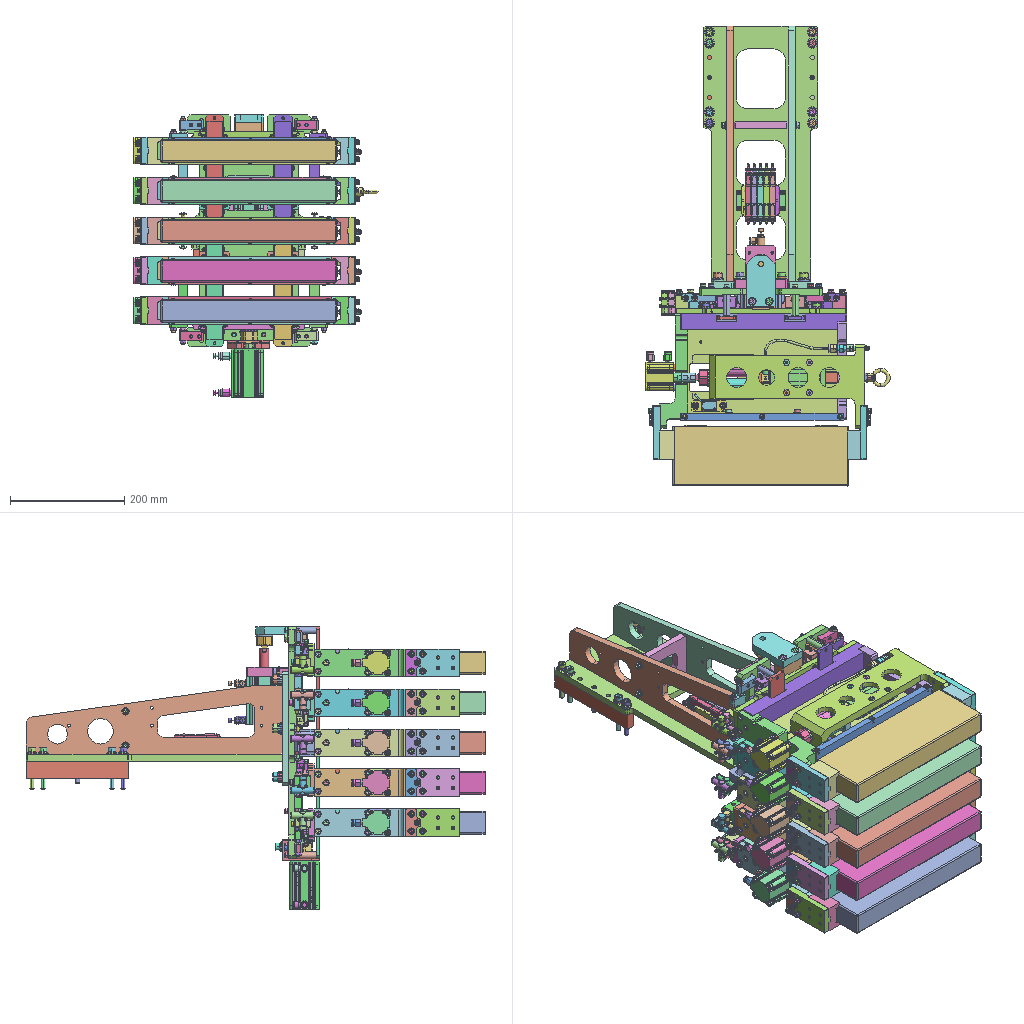Assembly | STEP file | 1222 different items | 1222 placed | box 427 x 805 x 495 mm
Parts list (item | name | quantity | parent item | size | volume), first 273 of 1222 items:
1 | 25A-CDQ2B32-15DZ-M9BWSDPC-Part-1 | x1 | in 25A-CDQ2B32-15DZ-M9BWSDPC | 27 x 4 x 4.6 mm | 354.995 mm3
2 | 25A-CDQ2B32-15DZ-M9BWSDPC-Part-1-1 | x1 | in 25A-CDQ2B32-15DZ-M9BWSDPC-1 | 27 x 4 x 4.6 mm | 354.995 mm3
3 | 25A-CDQ2B32-15DZ-M9BWSDPC-Part-1-2 | x1 | in 25A-CDQ2B32-15DZ-M9BWSDPC-2 | 27 x 4 x 4.6 mm | 354.995 mm3
4 | 25A-CDQ2B32-15DZ-M9BWSDPC-Part-1-3 | x1 | in 25A-CDQ2B32-15DZ-M9BWSDPC-3 | 27 x 4 x 4.6 mm | 354.995 mm3
5 | 25A-CDQ2B32-15DZ-M9BWSDPC-Part-1-4 | x1 | in 25A-CDQ2B32-15DZ-M9BWSDPC-4 | 27 x 4 x 4.6 mm | 354.995 mm3
6 | 25A-CDQ2B32-15DZ-M9BWSDPC-Part-2 | x1 | in 25A-CDQ2B32-15DZ-M9BWSDPC | 48 x 45 x 49.5 mm | 58108 mm3
7 | 25A-CDQ2B32-15DZ-M9BWSDPC-Part-2-1 | x1 | in 25A-CDQ2B32-15DZ-M9BWSDPC-1 | 48 x 45 x 49.5 mm | 58108 mm3
8 | 25A-CDQ2B32-15DZ-M9BWSDPC-Part-2-2 | x1 | in 25A-CDQ2B32-15DZ-M9BWSDPC-2 | 48 x 45 x 49.5 mm | 58108 mm3
9 | 25A-CDQ2B32-15DZ-M9BWSDPC-Part-2-3 | x1 | in 25A-CDQ2B32-15DZ-M9BWSDPC-3 | 48 x 45 x 49.5 mm | 58108 mm3
10 | 25A-CDQ2B32-15DZ-M9BWSDPC-Part-2-4 | x1 | in 25A-CDQ2B32-15DZ-M9BWSDPC-4 | 48 x 45 x 49.5 mm | 58108 mm3
11 | 25A-CDQ2B32-15DZ-M9BWSDPC-Part-3 | x1 | in 25A-CDQ2B32-15DZ-M9BWSDPC | 27 x 4 x 4.6 mm | 354.995 mm3
12 | 25A-CDQ2B32-15DZ-M9BWSDPC-Part-3-1 | x1 | in 25A-CDQ2B32-15DZ-M9BWSDPC-1 | 27 x 4 x 4.6 mm | 354.995 mm3
13 | 25A-CDQ2B32-15DZ-M9BWSDPC-Part-3-2 | x1 | in 25A-CDQ2B32-15DZ-M9BWSDPC-2 | 27 x 4 x 4.6 mm | 354.995 mm3
14 | 25A-CDQ2B32-15DZ-M9BWSDPC-Part-3-3 | x1 | in 25A-CDQ2B32-15DZ-M9BWSDPC-3 | 27 x 4 x 4.6 mm | 354.995 mm3
15 | 25A-CDQ2B32-15DZ-M9BWSDPC-Part-3-4 | x1 | in 25A-CDQ2B32-15DZ-M9BWSDPC-4 | 27 x 4 x 4.6 mm | 354.995 mm3
16 | 25A-CDQ2B40-45DZ-M9BWSDPC-Part-1 | x1 | in 25A-CDQ2B40-45DZ-M9BWSDPC | 84.5 x 52 x 57 mm | 122749 mm3
17 | 25A-CDQ2B40-45DZ-M9BWSDPC-Part-1-1 | x1 | in 25A-CDQ2B40-45DZ-M9BWSDPC-1 | 27 x 4 x 4.6 mm | 354.995 mm3
18 | 25A-CDQ2B40-45DZ-M9BWSDPC-Part-2 | x1 | in 25A-CDQ2B40-45DZ-M9BWSDPC | 27 x 4 x 4.6 mm | 354.995 mm3
19 | 25A-CDQ2B40-45DZ-M9BWSDPC-Part-2-1 | x1 | in 25A-CDQ2B40-45DZ-M9BWSDPC-1 | 27 x 4 x 4.6 mm | 354.995 mm3
20 | 25A-CDQ2B40-45DZ-M9BWSDPC-Part-3 | x1 | in 25A-CDQ2B40-45DZ-M9BWSDPC | 27 x 4 x 4.6 mm | 354.995 mm3
21 | 25A-CDQ2B40-45DZ-M9BWSDPC-Part-3-1 | x1 | in 25A-CDQ2B40-45DZ-M9BWSDPC-1 | 84.5 x 52 x 57 mm | 122749 mm3
22 | AS2002FG-06A | x1 | in elevator8 | 12.3 x 31.4 x 43.1 mm | 6190 mm3
23 | AS2002FG-06A-1 | x1 | in elevator8 | 12.3 x 31.4 x 43.1 mm | 6190 mm3
24 | AS2002FG-06A-2 | x1 | in elevator8 | 12.3 x 31.4 x 43.1 mm | 6190 mm3
25 | AS2002FG-06A-3 | x1 | in elevator8 | 12.3 x 31.4 x 43.1 mm | 6190 mm3
26 | AS2002FG-06A-4 | x1 | in elevator8 | 12.3 x 31.4 x 43.1 mm | 6190 mm3
27 | AS2002FG-06A-5 | x1 | in elevator8 | 12.3 x 31.4 x 43.1 mm | 6190 mm3
28 | AS2002FG-06A-6 | x1 | in elevator8 | 12.3 x 31.4 x 43.1 mm | 6190 mm3
29 | AS2002FG-06A-7 | x1 | in elevator8 | 12.3 x 31.4 x 43.1 mm | 6190 mm3
30 | AS2002FG-06A-8 | x1 | in elevator8 | 12.3 x 31.4 x 43.1 mm | 6190 mm3
31 | AS2002FG-06A-9 | x1 | in elevator8 | 12.3 x 31.4 x 43.1 mm | 6190 mm3
32 | AS2201FG-01-06S | x1 | in elevator8 | 14.2 x 35.2 x 27.5 mm | 4200 mm3
33 | AS2201FG-01-06S-1 | x1 | in elevator8 | 14.2 x 35.2 x 27.5 mm | 4200 mm3
34 | AS2201FG-01-06S-2 | x1 | in elevator8 | 14.2 x 35.2 x 27.5 mm | 4200 mm3
35 | AS2201FG-01-06S-3 | x1 | in elevator8 | 14.2 x 35.2 x 27.5 mm | 4200 mm3
36 | B-1132-8 | x1 | in elevator8 | 32.6 x 39.3 x 16 mm | 3782 mm3
37 | BB62-M10-30L | x1 | in J454-EBZ05-02-00 | 16 x 40 x 16 mm | 3957 mm3
38 | BB62-M10-30L-1 | x1 | in J454-EBZ05-02-00 | 16 x 40 x 16 mm | 3957 mm3
39 | BB62-M10-30L-2 | x1 | in J454-EBZ05-02-00 | 16 x 40 x 16 mm | 3957 mm3
40 | BB62-M10-30L-3 | x1 | in J454-EBZ05-02-00 | 16 x 40 x 16 mm | 3957 mm3
41 | BB62-M10-30L-4 | x1 | in J454-EBZ05-02-00 | 16 x 40 x 16 mm | 3957 mm3
42 | BB62-M10-30L-5 | x1 | in J454-EBZ05-02-00 | 16 x 40 x 16 mm | 3957 mm3
43 | BB62-M3-30L | x1 | in elevator8 | 5.5 x 33 x 5.5 mm | 272.045 mm3
44 | BB62-M3-30L-1 | x1 | in elevator8 | 5.5 x 33 x 5.5 mm | 272.045 mm3
45 | BB62-M3-30L-2 | x1 | in elevator8 | 5.5 x 33 x 5.5 mm | 272.045 mm3
46 | BB62-M3-30L-3 | x1 | in elevator8 | 5.5 x 33 x 5.5 mm | 272.045 mm3
47 | BB62-M3-30L-4 | x1 | in elevator8 | 5.5 x 33 x 5.5 mm | 272.045 mm3
48 | BB62-M3-30L-5 | x1 | in elevator8 | 5.5 x 33 x 5.5 mm | 272.045 mm3
49 | BB62-M3-30L-6 | x1 | in elevator8 | 5.5 x 33 x 5.5 mm | 272.045 mm3
50 | BB62-M3-30L-7 | x1 | in elevator8 | 5.5 x 33 x 5.5 mm | 272.045 mm3
51 | BB62-M3-40L | x1 | in elevator8 | 5.5 x 43 x 5.5 mm | 342.731 mm3
52 | BB62-M3-40L-1 | x1 | in elevator8 | 5.5 x 43 x 5.5 mm | 342.731 mm3
53 | BB62-M3-8L | x1 | in J454-EBZ05-18-00 | 5.5 x 11 x 5.5 mm | 116.536 mm3
54 | BB62-M3-8L-1 | x1 | in J454-EBZ05-18-00 | 5.5 x 11 x 5.5 mm | 116.536 mm3
55 | BB62-M3-8L-2 | x1 | in J454-EBZ05-18-00-1 | 5.5 x 11 x 5.5 mm | 116.536 mm3
56 | BB62-M3-8L-3 | x1 | in J454-EBZ05-18-00-1 | 5.5 x 11 x 5.5 mm | 116.536 mm3
57 | BB62-M3-8L-4 | x1 | in J454-EBZ05-18-00-2 | 5.5 x 11 x 5.5 mm | 116.536 mm3
58 | BB62-M3-8L-5 | x1 | in J454-EBZ05-18-00-2 | 5.5 x 11 x 5.5 mm | 116.536 mm3
59 | BB62-M3-8L-6 | x1 | in J454-EBZ05-18-00-3 | 5.5 x 11 x 5.5 mm | 116.536 mm3
60 | BB62-M3-8L-7 | x1 | in J454-EBZ05-18-00-3 | 5.5 x 11 x 5.5 mm | 116.536 mm3
61 | BB62-M3-8L-8 | x1 | in J454-EBZ05-18-00-4 | 5.5 x 11 x 5.5 mm | 116.536 mm3
62 | BB62-M3-8L-9 | x1 | in J454-EBZ05-18-00-4 | 5.5 x 11 x 5.5 mm | 116.536 mm3
63 | BB62-M4-12L | x1 | in J454-EBZ05-01-04 | 7 x 16 x 7 mm | 280.182 mm3
64 | BB62-M4-12L-1 | x1 | in J454-EBZ05-01-04 | 7 x 16 x 7 mm | 280.182 mm3
65 | BB62-M4-8L | x1 | in J454-EBZ05-37-04 | 7 x 12 x 7 mm | 229.916 mm3
66 | BB62-M4-8L-1 | x1 | in J454-EBZ05-37-04-1 | 7 x 12 x 7 mm | 229.916 mm3
67 | BB62-M4-8L-2 | x1 | in J454-EBZ05-37-04-2 | 7 x 12 x 7 mm | 229.916 mm3
68 | BB62-M4-8L-3 | x1 | in J454-EBZ05-37-04-3 | 7 x 12 x 7 mm | 229.916 mm3
69 | BB62-M4-8L-4 | x1 | in J454-EBZ05-37-04-4 | 7 x 12 x 7 mm | 229.916 mm3
70 | BB62-M4-8L-5 | x1 | in J454-EBZ05-37-04-5 | 7 x 12 x 7 mm | 229.916 mm3
71 | BB62-M4-8L-6 | x1 | in J454-EBZ05-37-04-6 | 7 x 12 x 7 mm | 229.916 mm3
72 | BB62-M4-8L-7 | x1 | in J454-EBZ05-37-04-7 | 7 x 12 x 7 mm | 229.916 mm3
73 | BB62-M4-8L-8 | x1 | in J454-EBZ05-37-04-8 | 7 x 12 x 7 mm | 229.916 mm3
74 | BB62-M4-8L-9 | x1 | in J454-EBZ05-37-04-9 | 7 x 12 x 7 mm | 229.916 mm3
75 | BB62-M5-12L | x1 | in J454-EBZ05-06-00 | 8.5 x 17 x 8.5 mm | 467.118 mm3
76 | BB62-M5-12L-1 | x1 | in J454-EBZ05-06-00 | 8.5 x 17 x 8.5 mm | 467.118 mm3
77 | BB62-M5-12L-2 | x1 | in J454-EBZ05-06-00 | 8.5 x 17 x 8.5 mm | 467.118 mm3
78 | BB62-M5-12L-3 | x1 | in J454-EBZ05-06-00 | 8.5 x 17 x 8.5 mm | 467.118 mm3
79 | BB62-M5-12L-4 | x1 | in J454-EBZ05-06-00 | 8.5 x 17 x 8.5 mm | 467.118 mm3
80 | BB62-M5-12L-5 | x1 | in J454-EBZ05-06-00 | 8.5 x 17 x 8.5 mm | 467.118 mm3
81 | BB62-M5-12L-6 | x1 | in J454-EBZ05-06-00 | 8.5 x 17 x 8.5 mm | 467.118 mm3
82 | BB62-M5-12L-7 | x1 | in J454-EBZ05-06-00 | 8.5 x 17 x 8.5 mm | 467.118 mm3
83 | BB62-M5-15L | x1 | in J454-EBZ05-17-00 | 8.5 x 20 x 8.5 mm | 526.023 mm3
84 | BB62-M5-15L-1 | x1 | in J454-EBZ05-17-00-1 | 8.5 x 20 x 8.5 mm | 526.023 mm3
85 | BB62-M5-15L-10 | x1 | in J454-EBZ05-12-03 | 8.5 x 20 x 8.5 mm | 526.023 mm3
86 | BB62-M5-15L-11 | x1 | in J454-EBZ05-17-00-2 | 8.5 x 20 x 8.5 mm | 526.023 mm3
87 | BB62-M5-15L-12 | x1 | in J454-EBZ05-17-00-3 | 8.5 x 20 x 8.5 mm | 526.023 mm3
88 | BB62-M5-15L-13 | x1 | in J454-EBZ05-17-00-4 | 8.5 x 20 x 8.5 mm | 526.023 mm3
89 | BB62-M5-15L-14 | x1 | in J454-EBZ05-17-00-5 | 8.5 x 20 x 8.5 mm | 526.023 mm3
90 | BB62-M5-15L-15 | x1 | in J454-EBZ05-12-03-1 | 8.5 x 20 x 8.5 mm | 526.023 mm3
91 | BB62-M5-15L-16 | x1 | in J454-EBZ05-12-03-1 | 8.5 x 20 x 8.5 mm | 526.023 mm3
92 | BB62-M5-15L-17 | x1 | in J454-EBZ05-12-03-1 | 8.5 x 20 x 8.5 mm | 526.023 mm3
93 | BB62-M5-15L-18 | x1 | in J454-EBZ05-12-03-1 | 8.5 x 20 x 8.5 mm | 526.023 mm3
94 | BB62-M5-15L-19 | x1 | in J454-EBZ05-12-03-1 | 8.5 x 20 x 8.5 mm | 526.023 mm3
95 | BB62-M5-15L-2 | x1 | in J454-EBZ05-12-03 | 8.5 x 20 x 8.5 mm | 526.023 mm3
96 | BB62-M5-15L-20 | x1 | in J454-EBZ05-12-03-1 | 8.5 x 20 x 8.5 mm | 526.023 mm3
97 | BB62-M5-15L-21 | x1 | in J454-EBZ05-12-03-1 | 8.5 x 20 x 8.5 mm | 526.023 mm3
98 | BB62-M5-15L-22 | x1 | in J454-EBZ05-12-03-1 | 8.5 x 20 x 8.5 mm | 526.023 mm3
99 | BB62-M5-15L-23 | x1 | in J454-EBZ05-12-03-1 | 8.5 x 20 x 8.5 mm | 526.023 mm3
100 | BB62-M5-15L-24 | x1 | in J454-EBZ05-17-00-6 | 8.5 x 20 x 8.5 mm | 526.023 mm3
101 | BB62-M5-15L-25 | x1 | in J454-EBZ05-17-00-7 | 8.5 x 20 x 8.5 mm | 526.023 mm3
102 | BB62-M5-15L-26 | x1 | in J454-EBZ05-22-00 | 8.5 x 20 x 8.5 mm | 526.023 mm3
103 | BB62-M5-15L-27 | x1 | in J454-EBZ05-22-00 | 8.5 x 20 x 8.5 mm | 526.023 mm3
104 | BB62-M5-15L-28 | x1 | in J454-EBZ05-22-00 | 8.5 x 20 x 8.5 mm | 526.023 mm3
105 | BB62-M5-15L-29 | x1 | in J454-EBZ05-22-00 | 8.5 x 20 x 8.5 mm | 526.023 mm3
106 | BB62-M5-15L-3 | x1 | in J454-EBZ05-12-03 | 8.5 x 20 x 8.5 mm | 526.023 mm3
107 | BB62-M5-15L-30 | x1 | in J454-EBZ05-22-00 | 8.5 x 20 x 8.5 mm | 526.023 mm3
108 | BB62-M5-15L-31 | x1 | in J454-EBZ05-22-00 | 8.5 x 20 x 8.5 mm | 526.023 mm3
109 | BB62-M5-15L-32 | x1 | in J454-EBZ05-22-00 | 8.5 x 20 x 8.5 mm | 526.023 mm3
110 | BB62-M5-15L-33 | x1 | in J454-EBZ05-22-00 | 8.5 x 20 x 8.5 mm | 526.023 mm3
111 | BB62-M5-15L-34 | x1 | in J454-EBZ05-26-00 | 8.5 x 20 x 8.5 mm | 526.023 mm3
112 | BB62-M5-15L-35 | x1 | in J454-EBZ05-26-00 | 8.5 x 20 x 8.5 mm | 526.023 mm3
113 | BB62-M5-15L-36 | x1 | in J454-EBZ05-26-00 | 8.5 x 20 x 8.5 mm | 526.023 mm3
114 | BB62-M5-15L-37 | x1 | in J454-EBZ05-26-00 | 8.5 x 20 x 8.5 mm | 526.023 mm3
115 | BB62-M5-15L-38 | x1 | in J454-EBZ05-26-00 | 8.5 x 20 x 8.5 mm | 526.023 mm3
116 | BB62-M5-15L-39 | x1 | in J454-EBZ05-26-00 | 8.5 x 20 x 8.5 mm | 526.023 mm3
117 | BB62-M5-15L-4 | x1 | in J454-EBZ05-12-03 | 8.5 x 20 x 8.5 mm | 526.023 mm3
118 | BB62-M5-15L-40 | x1 | in J454-EBZ05-26-00 | 8.5 x 20 x 8.5 mm | 526.023 mm3
119 | BB62-M5-15L-41 | x1 | in J454-EBZ05-26-00 | 8.5 x 20 x 8.5 mm | 526.023 mm3
120 | BB62-M5-15L-42 | x1 | in J454-EBZ05-17-00-8 | 8.5 x 20 x 8.5 mm | 526.023 mm3
121 | BB62-M5-15L-43 | x1 | in J454-EBZ05-17-00-9 | 8.5 x 20 x 8.5 mm | 526.023 mm3
122 | BB62-M5-15L-44 | x1 | in J454-EBZ05-17-00-10 | 8.5 x 20 x 8.5 mm | 526.023 mm3
123 | BB62-M5-15L-45 | x1 | in J454-EBZ05-17-00-11 | 8.5 x 20 x 8.5 mm | 526.023 mm3
124 | BB62-M5-15L-46 | x1 | in J454-EBZ05-12-03-2 | 8.5 x 20 x 8.5 mm | 526.023 mm3
125 | BB62-M5-15L-47 | x1 | in J454-EBZ05-12-03-2 | 8.5 x 20 x 8.5 mm | 526.023 mm3
126 | BB62-M5-15L-48 | x1 | in J454-EBZ05-12-03-2 | 8.5 x 20 x 8.5 mm | 526.023 mm3
127 | BB62-M5-15L-49 | x1 | in J454-EBZ05-12-03-2 | 8.5 x 20 x 8.5 mm | 526.023 mm3
128 | BB62-M5-15L-5 | x1 | in J454-EBZ05-12-03 | 8.5 x 20 x 8.5 mm | 526.023 mm3
129 | BB62-M5-15L-50 | x1 | in J454-EBZ05-12-03-2 | 8.5 x 20 x 8.5 mm | 526.023 mm3
130 | BB62-M5-15L-51 | x1 | in J454-EBZ05-12-03-2 | 8.5 x 20 x 8.5 mm | 526.023 mm3
131 | BB62-M5-15L-52 | x1 | in J454-EBZ05-12-03-2 | 8.5 x 20 x 8.5 mm | 526.023 mm3
132 | BB62-M5-15L-53 | x1 | in J454-EBZ05-12-03-2 | 8.5 x 20 x 8.5 mm | 526.023 mm3
133 | BB62-M5-15L-54 | x1 | in J454-EBZ05-12-03-2 | 8.5 x 20 x 8.5 mm | 526.023 mm3
134 | BB62-M5-15L-55 | x1 | in J454-EBZ05-17-00-12 | 8.5 x 20 x 8.5 mm | 526.023 mm3
135 | BB62-M5-15L-56 | x1 | in J454-EBZ05-17-00-13 | 8.5 x 20 x 8.5 mm | 526.023 mm3
136 | BB62-M5-15L-57 | x1 | in J454-EBZ05-12-03-3 | 8.5 x 20 x 8.5 mm | 526.023 mm3
137 | BB62-M5-15L-58 | x1 | in J454-EBZ05-12-03-3 | 8.5 x 20 x 8.5 mm | 526.023 mm3
138 | BB62-M5-15L-59 | x1 | in J454-EBZ05-12-03-3 | 8.5 x 20 x 8.5 mm | 526.023 mm3
139 | BB62-M5-15L-6 | x1 | in J454-EBZ05-12-03 | 8.5 x 20 x 8.5 mm | 526.023 mm3
140 | BB62-M5-15L-60 | x1 | in J454-EBZ05-12-03-3 | 8.5 x 20 x 8.5 mm | 526.023 mm3
141 | BB62-M5-15L-61 | x1 | in J454-EBZ05-12-03-3 | 8.5 x 20 x 8.5 mm | 526.023 mm3
142 | BB62-M5-15L-62 | x1 | in J454-EBZ05-12-03-3 | 8.5 x 20 x 8.5 mm | 526.023 mm3
143 | BB62-M5-15L-63 | x1 | in J454-EBZ05-12-03-3 | 8.5 x 20 x 8.5 mm | 526.023 mm3
144 | BB62-M5-15L-64 | x1 | in J454-EBZ05-12-03-3 | 8.5 x 20 x 8.5 mm | 526.023 mm3
145 | BB62-M5-15L-65 | x1 | in J454-EBZ05-12-03-3 | 8.5 x 20 x 8.5 mm | 526.023 mm3
146 | BB62-M5-15L-66 | x1 | in J454-EBZ05-17-00-14 | 8.5 x 20 x 8.5 mm | 526.023 mm3
147 | BB62-M5-15L-67 | x1 | in J454-EBZ05-17-00-15 | 8.5 x 20 x 8.5 mm | 526.023 mm3
148 | BB62-M5-15L-68 | x1 | in J454-EBZ05-22-00-1 | 8.5 x 20 x 8.5 mm | 526.023 mm3
149 | BB62-M5-15L-69 | x1 | in J454-EBZ05-22-00-1 | 8.5 x 20 x 8.5 mm | 526.023 mm3
150 | BB62-M5-15L-7 | x1 | in J454-EBZ05-12-03 | 8.5 x 20 x 8.5 mm | 526.023 mm3
151 | BB62-M5-15L-70 | x1 | in J454-EBZ05-22-00-1 | 8.5 x 20 x 8.5 mm | 526.023 mm3
152 | BB62-M5-15L-71 | x1 | in J454-EBZ05-22-00-1 | 8.5 x 20 x 8.5 mm | 526.023 mm3
153 | BB62-M5-15L-72 | x1 | in J454-EBZ05-22-00-1 | 8.5 x 20 x 8.5 mm | 526.023 mm3
154 | BB62-M5-15L-73 | x1 | in J454-EBZ05-22-00-1 | 8.5 x 20 x 8.5 mm | 526.023 mm3
155 | BB62-M5-15L-74 | x1 | in J454-EBZ05-22-00-1 | 8.5 x 20 x 8.5 mm | 526.023 mm3
156 | BB62-M5-15L-75 | x1 | in J454-EBZ05-22-00-1 | 8.5 x 20 x 8.5 mm | 526.023 mm3
157 | BB62-M5-15L-76 | x1 | in J454-EBZ05-26-00-1 | 8.5 x 20 x 8.5 mm | 526.023 mm3
158 | BB62-M5-15L-77 | x1 | in J454-EBZ05-26-00-1 | 8.5 x 20 x 8.5 mm | 526.023 mm3
159 | BB62-M5-15L-78 | x1 | in J454-EBZ05-26-00-1 | 8.5 x 20 x 8.5 mm | 526.023 mm3
160 | BB62-M5-15L-79 | x1 | in J454-EBZ05-26-00-1 | 8.5 x 20 x 8.5 mm | 526.023 mm3
161 | BB62-M5-15L-8 | x1 | in J454-EBZ05-12-03 | 8.5 x 20 x 8.5 mm | 526.023 mm3
162 | BB62-M5-15L-80 | x1 | in J454-EBZ05-26-00-1 | 8.5 x 20 x 8.5 mm | 526.023 mm3
163 | BB62-M5-15L-81 | x1 | in J454-EBZ05-26-00-1 | 8.5 x 20 x 8.5 mm | 526.023 mm3
164 | BB62-M5-15L-82 | x1 | in J454-EBZ05-26-00-1 | 8.5 x 20 x 8.5 mm | 526.023 mm3
165 | BB62-M5-15L-83 | x1 | in J454-EBZ05-26-00-1 | 8.5 x 20 x 8.5 mm | 526.023 mm3
166 | BB62-M5-15L-84 | x1 | in J454-EBZ05-17-00-16 | 8.5 x 20 x 8.5 mm | 526.023 mm3
167 | BB62-M5-15L-85 | x1 | in J454-EBZ05-17-00-17 | 8.5 x 20 x 8.5 mm | 526.023 mm3
168 | BB62-M5-15L-86 | x1 | in J454-EBZ05-12-03-4 | 8.5 x 20 x 8.5 mm | 526.023 mm3
169 | BB62-M5-15L-87 | x1 | in J454-EBZ05-12-03-4 | 8.5 x 20 x 8.5 mm | 526.023 mm3
170 | BB62-M5-15L-88 | x1 | in J454-EBZ05-12-03-4 | 8.5 x 20 x 8.5 mm | 526.023 mm3
171 | BB62-M5-15L-89 | x1 | in J454-EBZ05-12-03-4 | 8.5 x 20 x 8.5 mm | 526.023 mm3
172 | BB62-M5-15L-9 | x1 | in J454-EBZ05-12-03 | 8.5 x 20 x 8.5 mm | 526.023 mm3
173 | BB62-M5-15L-90 | x1 | in J454-EBZ05-12-03-4 | 8.5 x 20 x 8.5 mm | 526.023 mm3
174 | BB62-M5-15L-91 | x1 | in J454-EBZ05-12-03-4 | 8.5 x 20 x 8.5 mm | 526.023 mm3
175 | BB62-M5-15L-92 | x1 | in J454-EBZ05-12-03-4 | 8.5 x 20 x 8.5 mm | 526.023 mm3
176 | BB62-M5-15L-93 | x1 | in J454-EBZ05-12-03-4 | 8.5 x 20 x 8.5 mm | 526.023 mm3
177 | BB62-M5-15L-94 | x1 | in J454-EBZ05-12-03-4 | 8.5 x 20 x 8.5 mm | 526.023 mm3
178 | BB62-M5-15L-95 | x1 | in J454-EBZ05-17-00-18 | 8.5 x 20 x 8.5 mm | 526.023 mm3
179 | BB62-M5-15L-96 | x1 | in J454-EBZ05-17-00-19 | 8.5 x 20 x 8.5 mm | 526.023 mm3
180 | BB62-M5-20L | x1 | in J454-EBZ05-06-00 | 8.5 x 25 x 8.5 mm | 624.198 mm3
181 | BB62-M5-20L-1 | x1 | in J454-EBZ05-06-00 | 8.5 x 25 x 8.5 mm | 624.198 mm3
182 | BB62-M5-20L-2 | x1 | in J454-EBZ05-06-00 | 8.5 x 25 x 8.5 mm | 624.198 mm3
183 | BB62-M5-20L-3 | x1 | in J454-EBZ05-06-00 | 8.5 x 25 x 8.5 mm | 624.198 mm3
184 | BB62-M5-20L-4 | x1 | in J454-EBZ05-06-00 | 8.5 x 25 x 8.5 mm | 624.198 mm3
185 | BB62-M5-20L-5 | x1 | in J454-EBZ05-06-00 | 8.5 x 25 x 8.5 mm | 624.198 mm3
186 | BB62-M5-22L | x1 | in J454-EBZ05-18-00 | 8.5 x 27 x 8.5 mm | 663.468 mm3
187 | BB62-M5-22L-1 | x1 | in J454-EBZ05-18-00 | 8.5 x 27 x 8.5 mm | 663.468 mm3
188 | BB62-M5-22L-10 | x1 | in J454-EBZ05-18-00-1 | 8.5 x 27 x 8.5 mm | 663.468 mm3
189 | BB62-M5-22L-11 | x1 | in J454-EBZ05-18-00-1 | 8.5 x 27 x 8.5 mm | 663.468 mm3
190 | BB62-M5-22L-12 | x1 | in J454-EBZ05-19-00-1 | 8.5 x 27 x 8.5 mm | 663.468 mm3
191 | BB62-M5-22L-13 | x1 | in J454-EBZ05-19-00-1 | 8.5 x 27 x 8.5 mm | 663.468 mm3
192 | BB62-M5-22L-14 | x1 | in J454-EBZ05-19-00-1 | 8.5 x 27 x 8.5 mm | 663.468 mm3
193 | BB62-M5-22L-15 | x1 | in J454-EBZ05-19-00-1 | 8.5 x 27 x 8.5 mm | 663.468 mm3
194 | BB62-M5-22L-16 | x1 | in J454-EBZ05-36-04-1 | 8.5 x 27 x 8.5 mm | 663.468 mm3
195 | BB62-M5-22L-17 | x1 | in J454-EBZ05-36-04-1 | 8.5 x 27 x 8.5 mm | 663.468 mm3
196 | BB62-M5-22L-18 | x1 | in J454-EBZ05-36-04-1 | 8.5 x 27 x 8.5 mm | 663.468 mm3
197 | BB62-M5-22L-19 | x1 | in J454-EBZ05-36-04-1 | 8.5 x 27 x 8.5 mm | 663.468 mm3
198 | BB62-M5-22L-2 | x1 | in J454-EBZ05-19-00 | 8.5 x 27 x 8.5 mm | 663.468 mm3
199 | BB62-M5-22L-20 | x1 | in J454-EBZ05-36-04-2 | 8.5 x 27 x 8.5 mm | 663.468 mm3
200 | BB62-M5-22L-21 | x1 | in J454-EBZ05-36-04-2 | 8.5 x 27 x 8.5 mm | 663.468 mm3
201 | BB62-M5-22L-22 | x1 | in J454-EBZ05-36-04-2 | 8.5 x 27 x 8.5 mm | 663.468 mm3
202 | BB62-M5-22L-23 | x1 | in J454-EBZ05-36-04-2 | 8.5 x 27 x 8.5 mm | 663.468 mm3
203 | BB62-M5-22L-24 | x1 | in J454-EBZ05-18-00-2 | 8.5 x 27 x 8.5 mm | 663.468 mm3
204 | BB62-M5-22L-25 | x1 | in J454-EBZ05-18-00-2 | 8.5 x 27 x 8.5 mm | 663.468 mm3
205 | BB62-M5-22L-26 | x1 | in J454-EBZ05-19-00-2 | 8.5 x 27 x 8.5 mm | 663.468 mm3
206 | BB62-M5-22L-27 | x1 | in J454-EBZ05-19-00-2 | 8.5 x 27 x 8.5 mm | 663.468 mm3
207 | BB62-M5-22L-28 | x1 | in J454-EBZ05-19-00-2 | 8.5 x 27 x 8.5 mm | 663.468 mm3
208 | BB62-M5-22L-29 | x1 | in J454-EBZ05-19-00-2 | 8.5 x 27 x 8.5 mm | 663.468 mm3
209 | BB62-M5-22L-3 | x1 | in J454-EBZ05-19-00 | 8.5 x 27 x 8.5 mm | 663.468 mm3
210 | BB62-M5-22L-30 | x1 | in J454-EBZ05-18-00-3 | 8.5 x 27 x 8.5 mm | 663.468 mm3
211 | BB62-M5-22L-31 | x1 | in J454-EBZ05-18-00-3 | 8.5 x 27 x 8.5 mm | 663.468 mm3
212 | BB62-M5-22L-32 | x1 | in J454-EBZ05-19-00-3 | 8.5 x 27 x 8.5 mm | 663.468 mm3
213 | BB62-M5-22L-33 | x1 | in J454-EBZ05-19-00-3 | 8.5 x 27 x 8.5 mm | 663.468 mm3
214 | BB62-M5-22L-34 | x1 | in J454-EBZ05-19-00-3 | 8.5 x 27 x 8.5 mm | 663.468 mm3
215 | BB62-M5-22L-35 | x1 | in J454-EBZ05-19-00-3 | 8.5 x 27 x 8.5 mm | 663.468 mm3
216 | BB62-M5-22L-36 | x1 | in J454-EBZ05-36-04-3 | 8.5 x 27 x 8.5 mm | 663.468 mm3
217 | BB62-M5-22L-37 | x1 | in J454-EBZ05-36-04-3 | 8.5 x 27 x 8.5 mm | 663.468 mm3
218 | BB62-M5-22L-38 | x1 | in J454-EBZ05-36-04-3 | 8.5 x 27 x 8.5 mm | 663.468 mm3
219 | BB62-M5-22L-39 | x1 | in J454-EBZ05-36-04-3 | 8.5 x 27 x 8.5 mm | 663.468 mm3
220 | BB62-M5-22L-4 | x1 | in J454-EBZ05-19-00 | 8.5 x 27 x 8.5 mm | 663.468 mm3
221 | BB62-M5-22L-40 | x1 | in J454-EBZ05-18-00-4 | 8.5 x 27 x 8.5 mm | 663.468 mm3
222 | BB62-M5-22L-41 | x1 | in J454-EBZ05-18-00-4 | 8.5 x 27 x 8.5 mm | 663.468 mm3
223 | BB62-M5-22L-42 | x1 | in J454-EBZ05-19-00-4 | 8.5 x 27 x 8.5 mm | 663.468 mm3
224 | BB62-M5-22L-43 | x1 | in J454-EBZ05-19-00-4 | 8.5 x 27 x 8.5 mm | 663.468 mm3
225 | BB62-M5-22L-44 | x1 | in J454-EBZ05-19-00-4 | 8.5 x 27 x 8.5 mm | 663.468 mm3
226 | BB62-M5-22L-45 | x1 | in J454-EBZ05-19-00-4 | 8.5 x 27 x 8.5 mm | 663.468 mm3
227 | BB62-M5-22L-46 | x1 | in J454-EBZ05-36-04-4 | 8.5 x 27 x 8.5 mm | 663.468 mm3
228 | BB62-M5-22L-47 | x1 | in J454-EBZ05-36-04-4 | 8.5 x 27 x 8.5 mm | 663.468 mm3
229 | BB62-M5-22L-48 | x1 | in J454-EBZ05-36-04-4 | 8.5 x 27 x 8.5 mm | 663.468 mm3
230 | BB62-M5-22L-49 | x1 | in J454-EBZ05-36-04-4 | 8.5 x 27 x 8.5 mm | 663.468 mm3
231 | BB62-M5-22L-5 | x1 | in J454-EBZ05-19-00 | 8.5 x 27 x 8.5 mm | 663.468 mm3
232 | BB62-M5-22L-6 | x1 | in J454-EBZ05-36-04 | 8.5 x 27 x 8.5 mm | 663.468 mm3
233 | BB62-M5-22L-7 | x1 | in J454-EBZ05-36-04 | 8.5 x 27 x 8.5 mm | 663.468 mm3
234 | BB62-M5-22L-8 | x1 | in J454-EBZ05-36-04 | 8.5 x 27 x 8.5 mm | 663.468 mm3
235 | BB62-M5-22L-9 | x1 | in J454-EBZ05-36-04 | 8.5 x 27 x 8.5 mm | 663.468 mm3
236 | BB62-M5-35L | x1 | in J454-EBZ05-27-00 | 8.5 x 40 x 8.5 mm | 918.722 mm3
237 | BB62-M5-35L-1 | x1 | in J454-EBZ05-27-00 | 8.5 x 40 x 8.5 mm | 918.722 mm3
238 | BB62-M5-35L-2 | x1 | in J454-EBZ05-27-00-1 | 8.5 x 40 x 8.5 mm | 918.722 mm3
239 | BB62-M5-35L-3 | x1 | in J454-EBZ05-27-00-1 | 8.5 x 40 x 8.5 mm | 918.722 mm3
240 | BB62-M5-35L-4 | x1 | in J454-EBZ05-27-00-2 | 8.5 x 40 x 8.5 mm | 918.722 mm3
241 | BB62-M5-35L-5 | x1 | in J454-EBZ05-27-00-2 | 8.5 x 40 x 8.5 mm | 918.722 mm3
242 | BB62-M5-35L-6 | x1 | in J454-EBZ05-27-00-3 | 8.5 x 40 x 8.5 mm | 918.722 mm3
243 | BB62-M5-35L-7 | x1 | in J454-EBZ05-27-00-3 | 8.5 x 40 x 8.5 mm | 918.722 mm3
244 | BB62-M5-40L | x1 | in J454-EBZ05-15-00 | 8.5 x 45 x 8.5 mm | 1017 mm3
245 | BB62-M5-40L-1 | x1 | in J454-EBZ05-15-00 | 8.5 x 45 x 8.5 mm | 1017 mm3
246 | BB62-M5-40L-10 | x1 | in J454-EBZ05-15-00-2 | 8.5 x 45 x 8.5 mm | 1017 mm3
247 | BB62-M5-40L-11 | x1 | in J454-EBZ05-15-00-2 | 8.5 x 45 x 8.5 mm | 1017 mm3
248 | BB62-M5-40L-12 | x1 | in J454-EBZ05-31-03-1 | 8.5 x 45 x 8.5 mm | 1017 mm3
249 | BB62-M5-40L-13 | x1 | in J454-EBZ05-31-03-1 | 8.5 x 45 x 8.5 mm | 1017 mm3
250 | BB62-M5-40L-14 | x1 | in J454-EBZ05-31-03-1 | 8.5 x 45 x 8.5 mm | 1017 mm3
251 | BB62-M5-40L-2 | x1 | in J454-EBZ05-15-00 | 8.5 x 45 x 8.5 mm | 1017 mm3
252 | BB62-M5-40L-3 | x1 | in J454-EBZ05-15-00-1 | 8.5 x 45 x 8.5 mm | 1017 mm3
253 | BB62-M5-40L-4 | x1 | in J454-EBZ05-15-00-1 | 8.5 x 45 x 8.5 mm | 1017 mm3
254 | BB62-M5-40L-5 | x1 | in J454-EBZ05-15-00-1 | 8.5 x 45 x 8.5 mm | 1017 mm3
255 | BB62-M5-40L-6 | x1 | in J454-EBZ05-31-03 | 8.5 x 45 x 8.5 mm | 1017 mm3
256 | BB62-M5-40L-7 | x1 | in J454-EBZ05-31-03 | 8.5 x 45 x 8.5 mm | 1017 mm3
257 | BB62-M5-40L-8 | x1 | in J454-EBZ05-31-03 | 8.5 x 45 x 8.5 mm | 1017 mm3
258 | BB62-M5-40L-9 | x1 | in J454-EBZ05-15-00-2 | 8.5 x 45 x 8.5 mm | 1017 mm3
259 | BB62-M5-50L | x1 | in elevator8 | 8.5 x 55 x 8.5 mm | 1213 mm3
260 | BB62-M5-50L-1 | x1 | in elevator8 | 8.5 x 55 x 8.5 mm | 1213 mm3
261 | BB62-M5-50L-10 | x1 | in elevator8 | 8.5 x 55 x 8.5 mm | 1213 mm3
262 | BB62-M5-50L-11 | x1 | in elevator8 | 8.5 x 55 x 8.5 mm | 1213 mm3
263 | BB62-M5-50L-12 | x1 | in elevator8 | 8.5 x 55 x 8.5 mm | 1213 mm3
264 | BB62-M5-50L-13 | x1 | in elevator8 | 8.5 x 55 x 8.5 mm | 1213 mm3
265 | BB62-M5-50L-14 | x1 | in elevator8 | 8.5 x 55 x 8.5 mm | 1213 mm3
266 | BB62-M5-50L-15 | x1 | in elevator8 | 8.5 x 55 x 8.5 mm | 1213 mm3
267 | BB62-M5-50L-16 | x1 | in elevator8 | 8.5 x 55 x 8.5 mm | 1213 mm3
268 | BB62-M5-50L-17 | x1 | in elevator8 | 8.5 x 55 x 8.5 mm | 1213 mm3
269 | BB62-M5-50L-18 | x1 | in elevator8 | 8.5 x 55 x 8.5 mm | 1213 mm3
270 | BB62-M5-50L-19 | x1 | in elevator8 | 8.5 x 55 x 8.5 mm | 1213 mm3
271 | BB62-M5-50L-2 | x1 | in elevator8 | 8.5 x 55 x 8.5 mm | 1213 mm3
272 | BB62-M5-50L-3 | x1 | in elevator8 | 8.5 x 55 x 8.5 mm | 1213 mm3
273 | BB62-M5-50L-4 | x1 | in elevator8 | 8.5 x 55 x 8.5 mm | 1213 mm3